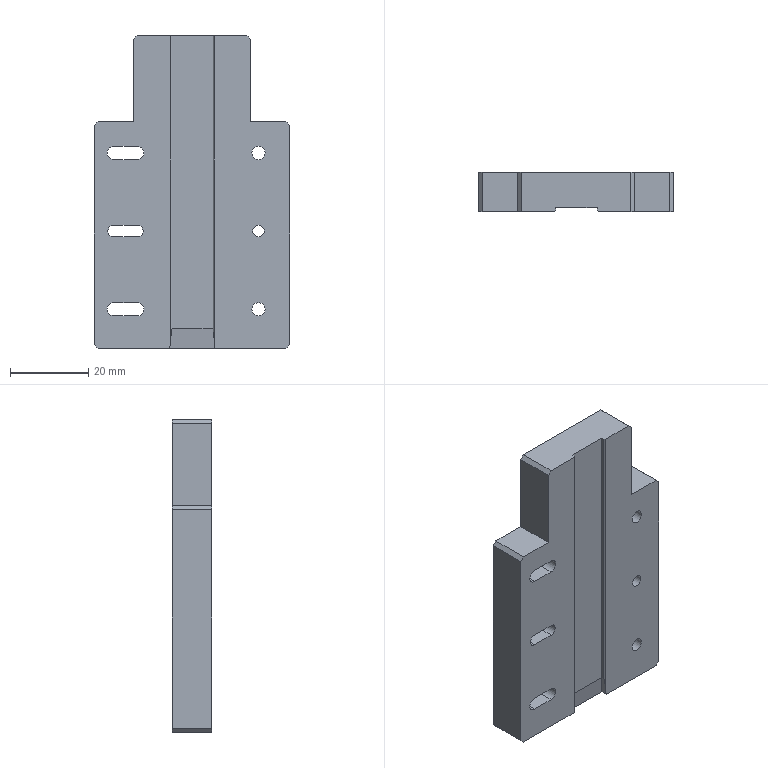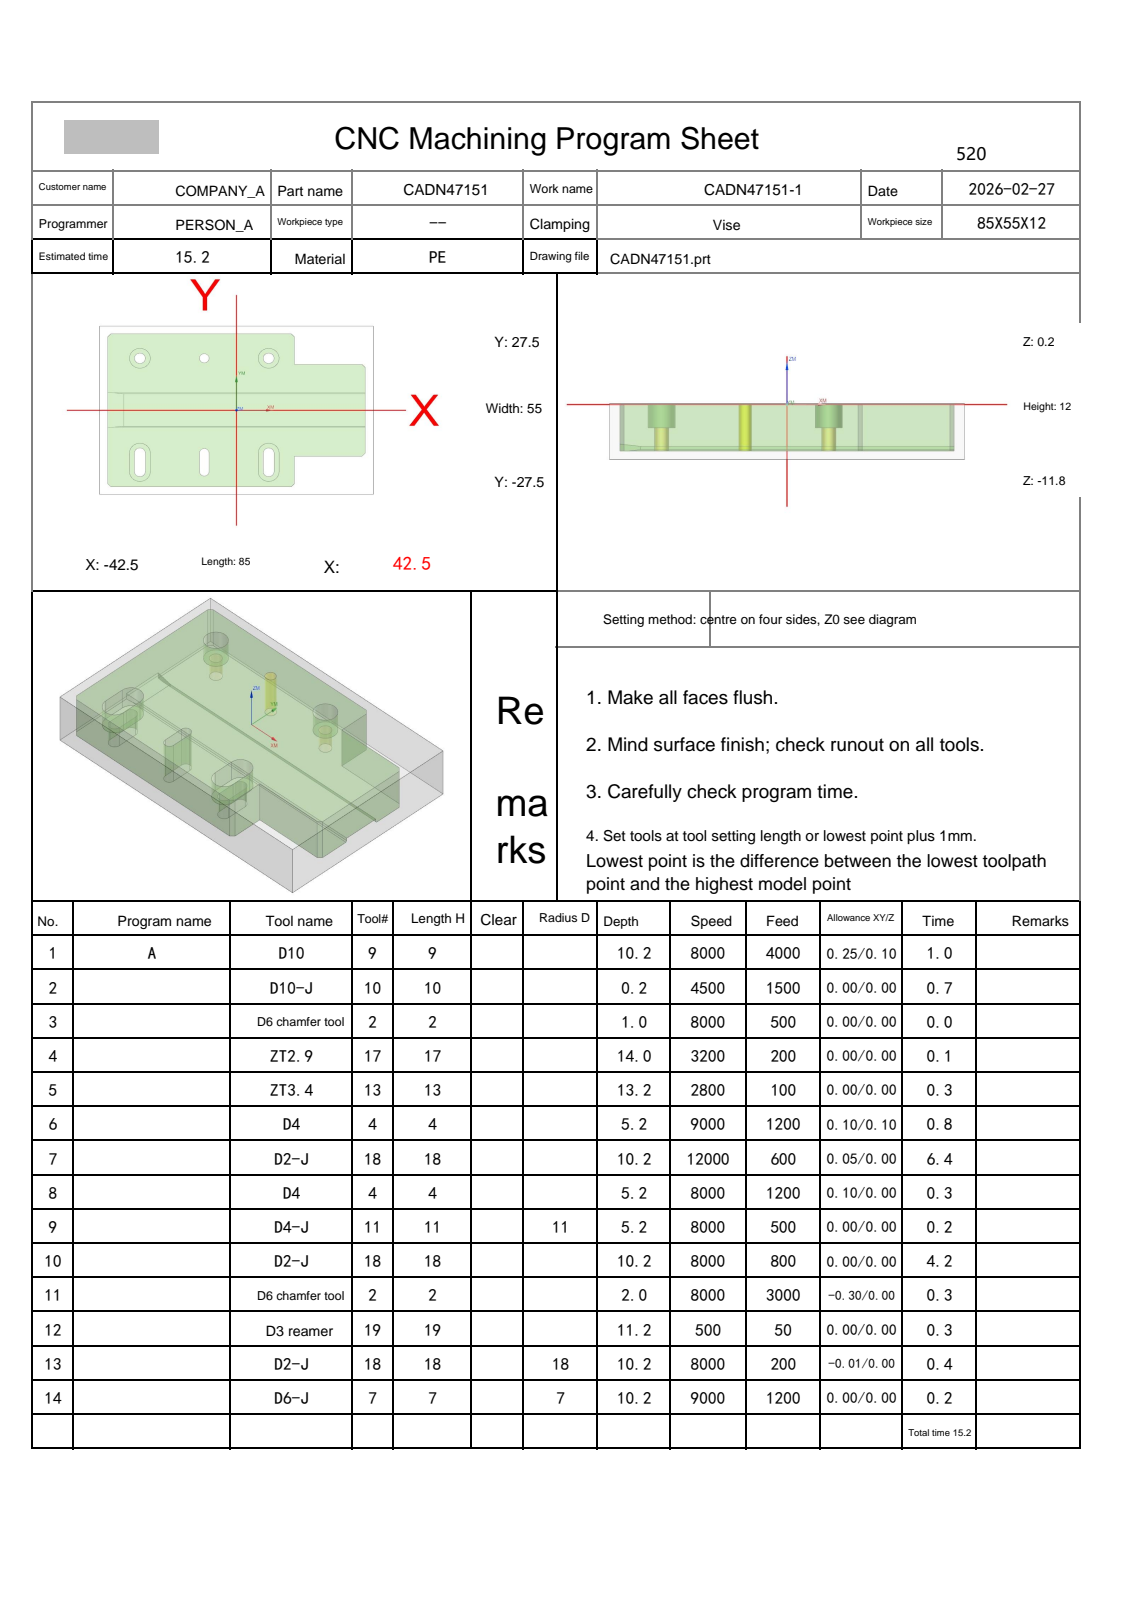NC program | NX | posted by the shop | part box 50 x 10 x 80 mm
Lines 1267 to 2934 of 8100, first 1180 of 1668 lines:
N7 T18 M06
(D2-J  D=2. R=0. H=18 ce=0.05 di=0.00)
G00 G90 G54 X-10.45 Y-17. M03 S12000
G43 H18 Z50.
M08
Z.5
G01 Y-20. Z.48 F600.
G03 X-10. Y-20.45 Z.475 I.45 J0.0
X-9.55 Y-20. Z.471 I0.0 J.45
G01 Y-14. Z.43
G03 X-10. Y-13.55 Z.426 I-.45 J0.0
X-10.45 Y-14. Z.421 I0.0 J-.45
G01 Y-20. Z.381
G03 X-10. Y-20.45 Z.376 I.45 J0.0
X-9.55 Y-20. Z.371 I0.0 J.45
G01 Y-14. Z.331
G03 X-10. Y-13.55 Z.327 I-.45 J0.0
X-10.45 Y-14. Z.322 I0.0 J-.45
G01 Y-20. Z.282
G03 X-10. Y-20.45 Z.277 I.45 J0.0
X-9.55 Y-20. Z.272 I0.0 J.45
G01 Y-14. Z.232
G03 X-10. Y-13.55 Z.228 I-.45 J0.0
X-10.45 Y-14. Z.223 I0.0 J-.45
G01 Y-20. Z.183
G03 X-10. Y-20.45 Z.178 I.45 J0.0
X-9.55 Y-20. Z.173 I0.0 J.45
G01 Y-14. Z.133
G03 X-10. Y-13.55 Z.129 I-.45 J0.0
X-10.45 Y-14. Z.124 I0.0 J-.45
G01 Y-20. Z.084
G03 X-10. Y-20.45 Z.079 I.45 J0.0
X-9.55 Y-20. Z.074 I0.0 J.45
G01 Y-14. Z.034
G03 X-10. Y-13.55 Z.029 I-.45 J0.0
X-10.45 Y-14. Z.025 I0.0 J-.45
G01 Y-20. Z-.015
G03 X-10. Y-20.45 Z-.02 I.45 J0.0
X-9.55 Y-20. Z-.025 I0.0 J.45
G01 Y-14. Z-.065
G03 X-10. Y-13.55 Z-.07 I-.45 J0.0
X-10.45 Y-14. Z-.074 I0.0 J-.45
G01 Y-20. Z-.114
G03 X-10. Y-20.45 Z-.119 I.45 J0.0
X-9.55 Y-20. Z-.124 I0.0 J.45
G01 Y-14. Z-.164
G03 X-10. Y-13.55 Z-.169 I-.45 J0.0
X-10.45 Y-14. Z-.173 I0.0 J-.45
G01 Y-20. Z-.213
G03 X-10. Y-20.45 Z-.218 I.45 J0.0
X-9.55 Y-20. Z-.223 I0.0 J.45
G01 Y-14. Z-.263
G03 X-10. Y-13.55 Z-.268 I-.45 J0.0
X-10.45 Y-14. Z-.272 I0.0 J-.45
G01 Y-20. Z-.312
G03 X-10. Y-20.45 Z-.317 I.45 J0.0
X-9.55 Y-20. Z-.322 I0.0 J.45
G01 Y-14. Z-.362
G03 X-10. Y-13.55 Z-.367 I-.45 J0.0
X-10.45 Y-14. Z-.371 I0.0 J-.45
G01 Y-20. Z-.412
G03 X-10. Y-20.45 Z-.416 I.45 J0.0
X-9.55 Y-20. Z-.421 I0.0 J.45
G01 Y-14. Z-.461
G03 X-10. Y-13.55 Z-.466 I-.45 J0.0
X-10.45 Y-14. Z-.471 I0.0 J-.45
G01 Y-20. Z-.511
G03 X-10. Y-20.45 Z-.515 I.45 J0.0
X-9.55 Y-20. Z-.52 I0.0 J.45
G01 Y-14. Z-.56
G03 X-10. Y-13.55 Z-.565 I-.45 J0.0
X-10.45 Y-14. Z-.57 I0.0 J-.45
G01 Y-20. Z-.61
G03 X-10. Y-20.45 Z-.614 I.45 J0.0
X-9.55 Y-20. Z-.619 I0.0 J.45
G01 Y-14. Z-.659
G03 X-10. Y-13.55 Z-.664 I-.45 J0.0
X-10.45 Y-14. Z-.669 I0.0 J-.45
G01 Y-20. Z-.709
G03 X-10. Y-20.45 Z-.713 I.45 J0.0
X-9.55 Y-20. Z-.718 I0.0 J.45
G01 Y-14. Z-.758
G03 X-10. Y-13.55 Z-.763 I-.45 J0.0
X-10.45 Y-14. Z-.768 I0.0 J-.45
G01 Y-20. Z-.808
G03 X-10. Y-20.45 Z-.813 I.45 J0.0
X-9.55 Y-20. Z-.817 I0.0 J.45
G01 Y-14. Z-.857
G03 X-10. Y-13.55 Z-.862 I-.45 J0.0
X-10.45 Y-14. Z-.867 I0.0 J-.45
G01 Y-20. Z-.907
G03 X-10. Y-20.45 Z-.912 I.45 J0.0
X-9.55 Y-20. Z-.916 I0.0 J.45
G01 Y-14. Z-.956
G03 X-10. Y-13.55 Z-.961 I-.45 J0.0
X-10.45 Y-14. Z-.966 I0.0 J-.45
G01 Y-20. Z-1.006
G03 X-10. Y-20.45 Z-1.011 I.45 J0.0
X-9.55 Y-20. Z-1.015 I0.0 J.45
G01 Y-14. Z-1.055
G03 X-10. Y-13.55 Z-1.06 I-.45 J0.0
X-10.45 Y-14. Z-1.065 I0.0 J-.45
G01 Y-20. Z-1.105
G03 X-10. Y-20.45 Z-1.11 I.45 J0.0
X-9.55 Y-20. Z-1.114 I0.0 J.45
G01 Y-14. Z-1.154
G03 X-10. Y-13.55 Z-1.159 I-.45 J0.0
X-10.45 Y-14. Z-1.164 I0.0 J-.45
G01 Y-20. Z-1.204
G03 X-10. Y-20.45 Z-1.209 I.45 J0.0
X-9.55 Y-20. Z-1.213 I0.0 J.45
G01 Y-14. Z-1.254
G03 X-10. Y-13.55 Z-1.258 I-.45 J0.0
X-10.45 Y-14. Z-1.263 I0.0 J-.45
G01 Y-20. Z-1.303
G03 X-10. Y-20.45 Z-1.308 I.45 J0.0
X-9.55 Y-20. Z-1.313 I0.0 J.45
G01 Y-14. Z-1.353
G03 X-10. Y-13.55 Z-1.357 I-.45 J0.0
X-10.45 Y-14. Z-1.362 I0.0 J-.45
G01 Y-20. Z-1.402
G03 X-10. Y-20.45 Z-1.407 I.45 J0.0
X-9.55 Y-20. Z-1.412 I0.0 J.45
G01 Y-14. Z-1.452
G03 X-10. Y-13.55 Z-1.456 I-.45 J0.0
X-10.45 Y-14. Z-1.461 I0.0 J-.45
G01 Y-20. Z-1.501
G03 X-10. Y-20.45 Z-1.506 I.45 J0.0
X-9.55 Y-20. Z-1.511 I0.0 J.45
G01 Y-14. Z-1.551
G03 X-10. Y-13.55 Z-1.555 I-.45 J0.0
X-10.45 Y-14. Z-1.56 I0.0 J-.45
G01 Y-20. Z-1.6
G03 X-10. Y-20.45 Z-1.605 I.45 J0.0
X-9.55 Y-20. Z-1.61 I0.0 J.45
G01 Y-14. Z-1.65
G03 X-10. Y-13.55 Z-1.654 I-.45 J0.0
X-10.45 Y-14. Z-1.659 I0.0 J-.45
G01 Y-20. Z-1.699
G03 X-10. Y-20.45 Z-1.704 I.45 J0.0
X-9.55 Y-20. Z-1.709 I0.0 J.45
G01 Y-14. Z-1.749
G03 X-10. Y-13.55 Z-1.754 I-.45 J0.0
X-10.45 Y-14. Z-1.758 I0.0 J-.45
G01 Y-20. Z-1.798
G03 X-10. Y-20.45 Z-1.803 I.45 J0.0
X-9.55 Y-20. Z-1.808 I0.0 J.45
G01 Y-14. Z-1.848
G03 X-10. Y-13.55 Z-1.853 I-.45 J0.0
X-10.45 Y-14. Z-1.857 I0.0 J-.45
G01 Y-20. Z-1.897
G03 X-10. Y-20.45 Z-1.902 I.45 J0.0
X-9.55 Y-20. Z-1.907 I0.0 J.45
G01 Y-14. Z-1.947
G03 X-10. Y-13.55 Z-1.952 I-.45 J0.0
X-10.45 Y-14. Z-1.956 I0.0 J-.45
G01 Y-20. Z-1.996
G03 X-10. Y-20.45 Z-2.001 I.45 J0.0
X-9.55 Y-20. Z-2.006 I0.0 J.45
G01 Y-14. Z-2.046
G03 X-10. Y-13.55 Z-2.051 I-.45 J0.0
X-10.45 Y-14. Z-2.055 I0.0 J-.45
G01 Y-20. Z-2.096
G03 X-10. Y-20.45 Z-2.1 I.45 J0.0
X-9.55 Y-20. Z-2.105 I0.0 J.45
G01 Y-14. Z-2.145
G03 X-10. Y-13.55 Z-2.15 I-.45 J0.0
X-10.45 Y-14. Z-2.154 I0.0 J-.45
G01 Y-20. Z-2.195
G03 X-10. Y-20.45 Z-2.199 I.45 J0.0
X-9.55 Y-20. Z-2.204 I0.0 J.45
G01 Y-14. Z-2.244
G03 X-10. Y-13.55 Z-2.249 I-.45 J0.0
X-10.45 Y-14. Z-2.254 I0.0 J-.45
G01 Y-20. Z-2.294
G03 X-10. Y-20.45 Z-2.298 I.45 J0.0
X-9.55 Y-20. Z-2.303 I0.0 J.45
G01 Y-14. Z-2.343
G03 X-10. Y-13.55 Z-2.348 I-.45 J0.0
X-10.45 Y-14. Z-2.353 I0.0 J-.45
G01 Y-20. Z-2.393
G03 X-10. Y-20.45 Z-2.397 I.45 J0.0
X-9.55 Y-20. Z-2.402 I0.0 J.45
G01 Y-14. Z-2.442
G03 X-10. Y-13.55 Z-2.447 I-.45 J0.0
X-10.45 Y-14. Z-2.452 I0.0 J-.45
G01 Y-20. Z-2.492
G03 X-10. Y-20.45 Z-2.496 I.45 J0.0
X-9.55 Y-20. Z-2.501 I0.0 J.45
G01 Y-14. Z-2.541
G03 X-10. Y-13.55 Z-2.546 I-.45 J0.0
X-10.45 Y-14. Z-2.551 I0.0 J-.45
G01 Y-20. Z-2.591
G03 X-10. Y-20.45 Z-2.596 I.45 J0.0
X-9.55 Y-20. Z-2.6 I0.0 J.45
G01 Y-14. Z-2.64
G03 X-10. Y-13.55 Z-2.645 I-.45 J0.0
X-10.45 Y-14. Z-2.65 I0.0 J-.45
G01 Y-20. Z-2.69
G03 X-10. Y-20.45 Z-2.695 I.45 J0.0
X-9.55 Y-20. Z-2.699 I0.0 J.45
G01 Y-14. Z-2.739
G03 X-10. Y-13.55 Z-2.744 I-.45 J0.0
X-10.45 Y-14. Z-2.749 I0.0 J-.45
G01 Y-20. Z-2.789
G03 X-10. Y-20.45 Z-2.794 I.45 J0.0
X-9.55 Y-20. Z-2.798 I0.0 J.45
G01 Y-14. Z-2.838
G03 X-10. Y-13.55 Z-2.843 I-.45 J0.0
X-10.45 Y-14. Z-2.848 I0.0 J-.45
G01 Y-20. Z-2.888
G03 X-10. Y-20.45 Z-2.893 I.45 J0.0
X-9.55 Y-20. Z-2.897 I0.0 J.45
G01 Y-14. Z-2.937
G03 X-10. Y-13.55 Z-2.942 I-.45 J0.0
X-10.45 Y-14. Z-2.947 I0.0 J-.45
G01 Y-20. Z-2.987
G03 X-10. Y-20.45 Z-2.992 I.45 J0.0
X-9.55 Y-20. Z-2.996 I0.0 J.45
G01 Y-14. Z-3.037
G03 X-10. Y-13.55 Z-3.041 I-.45 J0.0
X-10.45 Y-14. Z-3.046 I0.0 J-.45
G01 Y-20. Z-3.086
G03 X-10. Y-20.45 Z-3.091 I.45 J0.0
X-9.55 Y-20. Z-3.096 I0.0 J.45
G01 Y-14. Z-3.136
G03 X-10. Y-13.55 Z-3.14 I-.45 J0.0
X-10.45 Y-14. Z-3.145 I0.0 J-.45
G01 Y-20. Z-3.185
G03 X-10. Y-20.45 Z-3.19 I.45 J0.0
X-9.55 Y-20. Z-3.195 I0.0 J.45
G01 Y-14. Z-3.235
G03 X-10. Y-13.55 Z-3.239 I-.45 J0.0
X-10.45 Y-14. Z-3.244 I0.0 J-.45
G01 Y-20. Z-3.284
G03 X-10. Y-20.45 Z-3.289 I.45 J0.0
X-9.55 Y-20. Z-3.294 I0.0 J.45
G01 Y-14. Z-3.334
G03 X-10. Y-13.55 Z-3.338 I-.45 J0.0
X-10.45 Y-14. Z-3.343 I0.0 J-.45
G01 Y-20. Z-3.383
G03 X-10. Y-20.45 Z-3.388 I.45 J0.0
X-9.55 Y-20. Z-3.393 I0.0 J.45
G01 Y-14. Z-3.433
G03 X-10. Y-13.55 Z-3.438 I-.45 J0.0
X-10.45 Y-14. Z-3.442 I0.0 J-.45
G01 Y-20. Z-3.482
G03 X-10. Y-20.45 Z-3.487 I.45 J0.0
X-9.55 Y-20. Z-3.492 I0.0 J.45
G01 Y-14. Z-3.532
G03 X-10. Y-13.55 Z-3.537 I-.45 J0.0
X-10.45 Y-14. Z-3.541 I0.0 J-.45
G01 Y-20. Z-3.581
G03 X-10. Y-20.45 Z-3.586 I.45 J0.0
X-9.55 Y-20. Z-3.591 I0.0 J.45
G01 Y-14. Z-3.631
G03 X-10. Y-13.55 Z-3.636 I-.45 J0.0
X-10.45 Y-14. Z-3.64 I0.0 J-.45
G01 Y-20. Z-3.68
G03 X-10. Y-20.45 Z-3.685 I.45 J0.0
X-9.55 Y-20. Z-3.69 I0.0 J.45
G01 Y-14. Z-3.73
G03 X-10. Y-13.55 Z-3.735 I-.45 J0.0
X-10.45 Y-14. Z-3.739 I0.0 J-.45
G01 Y-20. Z-3.779
G03 X-10. Y-20.45 Z-3.784 I.45 J0.0
X-9.55 Y-20. Z-3.789 I0.0 J.45
G01 Y-14. Z-3.829
G03 X-10. Y-13.55 Z-3.834 I-.45 J0.0
X-10.45 Y-14. Z-3.838 I0.0 J-.45
G01 Y-20. Z-3.879
G03 X-10. Y-20.45 Z-3.883 I.45 J0.0
X-9.55 Y-20. Z-3.888 I0.0 J.45
G01 Y-14. Z-3.928
G03 X-10. Y-13.55 Z-3.933 I-.45 J0.0
X-10.45 Y-14. Z-3.938 I0.0 J-.45
G01 Y-20. Z-3.978
G03 X-10. Y-20.45 Z-3.982 I.45 J0.0
X-9.55 Y-20. Z-3.987 I0.0 J.45
G01 Y-14. Z-4.027
G03 X-10. Y-13.55 Z-4.032 I-.45 J0.0
X-10.45 Y-14. Z-4.037 I0.0 J-.45
G01 Y-20. Z-4.077
G03 X-10. Y-20.45 Z-4.081 I.45 J0.0
X-9.55 Y-20. Z-4.086 I0.0 J.45
G01 Y-14. Z-4.126
G03 X-10. Y-13.55 Z-4.131 I-.45 J0.0
X-10.45 Y-14. Z-4.136 I0.0 J-.45
G01 Y-20. Z-4.176
G03 X-10. Y-20.45 Z-4.18 I.45 J0.0
X-9.55 Y-20. Z-4.185 I0.0 J.45
G01 Y-14. Z-4.225
G03 X-10. Y-13.55 Z-4.23 I-.45 J0.0
X-10.45 Y-14. Z-4.235 I0.0 J-.45
G01 Y-20. Z-4.275
G03 X-10. Y-20.45 Z-4.279 I.45 J0.0
X-9.55 Y-20. Z-4.284 I0.0 J.45
G01 Y-14. Z-4.324
G03 X-10. Y-13.55 Z-4.329 I-.45 J0.0
X-10.45 Y-14. Z-4.334 I0.0 J-.45
G01 Y-20. Z-4.374
G03 X-10. Y-20.45 Z-4.379 I.45 J0.0
X-9.55 Y-20. Z-4.383 I0.0 J.45
G01 Y-14. Z-4.423
G03 X-10. Y-13.55 Z-4.428 I-.45 J0.0
X-10.45 Y-14. Z-4.433 I0.0 J-.45
G01 Y-20. Z-4.473
G03 X-10. Y-20.45 Z-4.478 I.45 J0.0
X-9.55 Y-20. Z-4.482 I0.0 J.45
G01 Y-14. Z-4.522
G03 X-10. Y-13.55 Z-4.527 I-.45 J0.0
X-10.45 Y-14. Z-4.532 I0.0 J-.45
G01 Y-20. Z-4.572
G03 X-10. Y-20.45 Z-4.577 I.45 J0.0
X-9.55 Y-20. Z-4.581 I0.0 J.45
G01 Y-14. Z-4.621
G03 X-10. Y-13.55 Z-4.626 I-.45 J0.0
X-10.45 Y-14. Z-4.631 I0.0 J-.45
G01 Y-20. Z-4.671
G03 X-10. Y-20.45 Z-4.676 I.45 J0.0
X-9.55 Y-20. Z-4.68 I0.0 J.45
G01 Y-14. Z-4.721
G03 X-10. Y-13.55 Z-4.725 I-.45 J0.0
X-10.45 Y-14. Z-4.73 I0.0 J-.45
G01 Y-20. Z-4.77
G03 X-10. Y-20.45 Z-4.775 I.45 J0.0
X-9.55 Y-20. Z-4.779 I0.0 J.45
G01 Y-14. Z-4.82
G03 X-10. Y-13.55 Z-4.824 I-.45 J0.0
X-10.45 Y-14. Z-4.829 I0.0 J-.45
G01 Y-20. Z-4.869
G03 X-10. Y-20.45 Z-4.874 I.45 J0.0
X-9.55 Y-20. Z-4.879 I0.0 J.45
G01 Y-14. Z-4.919
G03 X-10. Y-13.55 Z-4.923 I-.45 J0.0
X-10.45 Y-14. Z-4.928 I0.0 J-.45
G01 Y-20. Z-4.968
G03 X-10. Y-20.45 Z-4.973 I.45 J0.0
X-9.55 Y-20. Z-4.978 I0.0 J.45
G01 Y-14. Z-5.018
G03 X-10. Y-13.55 Z-5.022 I-.45 J0.0
X-10.45 Y-14. Z-5.027 I0.0 J-.45
G01 Y-20. Z-5.067
G03 X-10. Y-20.45 Z-5.072 I.45 J0.0
X-9.55 Y-20. Z-5.077 I0.0 J.45
G01 Y-14. Z-5.117
G03 X-10. Y-13.55 Z-5.121 I-.45 J0.0
X-10.45 Y-14. Z-5.126 I0.0 J-.45
G01 Y-20. Z-5.166
G03 X-10. Y-20.45 Z-5.171 I.45 J0.0
X-9.55 Y-20. Z-5.176 I0.0 J.45
G01 Y-14. Z-5.216
G03 X-10. Y-13.55 Z-5.221 I-.45 J0.0
X-10.45 Y-14. Z-5.225 I0.0 J-.45
G01 Y-20. Z-5.265
G03 X-10. Y-20.45 Z-5.27 I.45 J0.0
X-9.55 Y-20. Z-5.275 I0.0 J.45
G01 Y-14. Z-5.315
G03 X-10. Y-13.55 Z-5.32 I-.45 J0.0
X-10.45 Y-14. Z-5.324 I0.0 J-.45
G01 Y-20. Z-5.364
G03 X-10. Y-20.45 Z-5.369 I.45 J0.0
X-9.55 Y-20. Z-5.374 I0.0 J.45
G01 Y-14. Z-5.414
G03 X-10. Y-13.55 Z-5.419 I-.45 J0.0
X-10.45 Y-14. Z-5.423 I0.0 J-.45
G01 Y-20. Z-5.463
G03 X-10. Y-20.45 Z-5.468 I.45 J0.0
X-9.55 Y-20. Z-5.473 I0.0 J.45
G01 Y-14. Z-5.513
G03 X-10. Y-13.55 Z-5.518 I-.45 J0.0
X-10.45 Y-14. Z-5.522 I0.0 J-.45
G01 Y-20. Z-5.562
G03 X-10. Y-20.45 Z-5.567 I.45 J0.0
X-9.55 Y-20. Z-5.572 I0.0 J.45
G01 Y-14. Z-5.612
G03 X-10. Y-13.55 Z-5.617 I-.45 J0.0
X-10.45 Y-14. Z-5.621 I0.0 J-.45
G01 Y-20. Z-5.662
G03 X-10. Y-20.45 Z-5.666 I.45 J0.0
X-9.55 Y-20. Z-5.671 I0.0 J.45
G01 Y-14. Z-5.711
G03 X-10. Y-13.55 Z-5.716 I-.45 J0.0
X-10.45 Y-14. Z-5.721 I0.0 J-.45
G01 Y-20. Z-5.761
G03 X-10. Y-20.45 Z-5.765 I.45 J0.0
X-9.55 Y-20. Z-5.77 I0.0 J.45
G01 Y-14. Z-5.81
G03 X-10. Y-13.55 Z-5.815 I-.45 J0.0
X-10.45 Y-14. Z-5.82 I0.0 J-.45
G01 Y-20. Z-5.86
G03 X-10. Y-20.45 Z-5.864 I.45 J0.0
X-9.55 Y-20. Z-5.869 I0.0 J.45
G01 Y-14. Z-5.909
G03 X-10. Y-13.55 Z-5.914 I-.45 J0.0
X-10.45 Y-14. Z-5.919 I0.0 J-.45
G01 Y-20. Z-5.959
G03 X-10. Y-20.45 Z-5.963 I.45 J0.0
X-9.55 Y-20. Z-5.968 I0.0 J.45
G01 Y-14. Z-6.008
G03 X-10. Y-13.55 Z-6.013 I-.45 J0.0
X-10.45 Y-14. Z-6.018 I0.0 J-.45
G01 Y-20. Z-6.058
G03 X-10. Y-20.45 Z-6.063 I.45 J0.0
X-9.55 Y-20. Z-6.067 I0.0 J.45
G01 Y-14. Z-6.107
G03 X-10. Y-13.55 Z-6.112 I-.45 J0.0
X-10.45 Y-14. Z-6.117 I0.0 J-.45
G01 Y-20. Z-6.157
G03 X-10. Y-20.45 Z-6.162 I.45 J0.0
X-9.55 Y-20. Z-6.166 I0.0 J.45
G01 Y-14. Z-6.206
G03 X-10. Y-13.55 Z-6.211 I-.45 J0.0
X-10.45 Y-14. Z-6.216 I0.0 J-.45
G01 Y-20. Z-6.256
G03 X-10. Y-20.45 Z-6.261 I.45 J0.0
X-9.55 Y-20. Z-6.265 I0.0 J.45
G01 Y-14. Z-6.305
G03 X-10. Y-13.55 Z-6.31 I-.45 J0.0
X-10.45 Y-14. Z-6.315 I0.0 J-.45
G01 Y-20. Z-6.355
G03 X-10. Y-20.45 Z-6.36 I.45 J0.0
X-9.55 Y-20. Z-6.364 I0.0 J.45
G01 Y-14. Z-6.404
G03 X-10. Y-13.55 Z-6.409 I-.45 J0.0
X-10.45 Y-14. Z-6.414 I0.0 J-.45
G01 Y-20. Z-6.454
G03 X-10. Y-20.45 Z-6.459 I.45 J0.0
X-9.55 Y-20. Z-6.463 I0.0 J.45
G01 Y-14. Z-6.504
G03 X-10. Y-13.55 Z-6.508 I-.45 J0.0
X-10.45 Y-14. Z-6.513 I0.0 J-.45
G01 Y-20. Z-6.553
G03 X-10. Y-20.45 Z-6.558 I.45 J0.0
X-9.55 Y-20. Z-6.563 I0.0 J.45
G01 Y-14. Z-6.603
G03 X-10. Y-13.55 Z-6.607 I-.45 J0.0
X-10.45 Y-14. Z-6.612 I0.0 J-.45
G01 Y-20. Z-6.652
G03 X-10. Y-20.45 Z-6.657 I.45 J0.0
X-9.55 Y-20. Z-6.662 I0.0 J.45
G01 Y-14. Z-6.702
G03 X-10. Y-13.55 Z-6.706 I-.45 J0.0
X-10.45 Y-14. Z-6.711 I0.0 J-.45
G01 Y-20. Z-6.751
G03 X-10. Y-20.45 Z-6.756 I.45 J0.0
X-9.55 Y-20. Z-6.761 I0.0 J.45
G01 Y-14. Z-6.801
G03 X-10. Y-13.55 Z-6.805 I-.45 J0.0
X-10.45 Y-14. Z-6.81 I0.0 J-.45
G01 Y-20. Z-6.85
G03 X-10. Y-20.45 Z-6.855 I.45 J0.0
X-9.55 Y-20. Z-6.86 I0.0 J.45
G01 Y-14. Z-6.9
G03 X-10. Y-13.55 Z-6.904 I-.45 J0.0
X-10.45 Y-14. Z-6.909 I0.0 J-.45
G01 Y-20. Z-6.949
G03 X-10. Y-20.45 Z-6.954 I.45 J0.0
X-9.55 Y-20. Z-6.959 I0.0 J.45
G01 Y-14. Z-6.999
G03 X-10. Y-13.55 Z-7.004 I-.45 J0.0
X-10.45 Y-14. Z-7.008 I0.0 J-.45
G01 Y-20. Z-7.048
G03 X-10. Y-20.45 Z-7.053 I.45 J0.0
X-9.55 Y-20. Z-7.058 I0.0 J.45
G01 Y-14. Z-7.098
G03 X-10. Y-13.55 Z-7.103 I-.45 J0.0
X-10.45 Y-14. Z-7.107 I0.0 J-.45
G01 Y-20. Z-7.147
G03 X-10. Y-20.45 Z-7.152 I.45 J0.0
X-9.55 Y-20. Z-7.157 I0.0 J.45
G01 Y-14. Z-7.197
G03 X-10. Y-13.55 Z-7.202 I-.45 J0.0
X-10.45 Y-14. Z-7.206 I0.0 J-.45
G01 Y-20. Z-7.246
G03 X-10. Y-20.45 Z-7.251 I.45 J0.0
X-9.55 Y-20. Z-7.256 I0.0 J.45
G01 Y-14. Z-7.296
G03 X-10. Y-13.55 Z-7.301 I-.45 J0.0
X-10.45 Y-14. Z-7.305 I0.0 J-.45
G01 Y-20. Z-7.346
G03 X-10. Y-20.45 Z-7.35 I.45 J0.0
X-9.55 Y-20. Z-7.355 I0.0 J.45
G01 Y-14. Z-7.395
G03 X-10. Y-13.55 Z-7.4 I-.45 J0.0
X-10.45 Y-14. Z-7.404 I0.0 J-.45
G01 Y-20. Z-7.445
G03 X-10. Y-20.45 Z-7.449 I.45 J0.0
X-9.55 Y-20. Z-7.454 I0.0 J.45
G01 Y-14. Z-7.494
G03 X-10. Y-13.55 Z-7.499 I-.45 J0.0
X-10.45 Y-14. Z-7.504 I0.0 J-.45
G01 Y-20. Z-7.544
G03 X-10. Y-20.45 Z-7.548 I.45 J0.0
X-9.55 Y-20. Z-7.553 I0.0 J.45
G01 Y-14. Z-7.593
G03 X-10. Y-13.55 Z-7.598 I-.45 J0.0
X-10.45 Y-14. Z-7.603 I0.0 J-.45
G01 Y-20. Z-7.643
G03 X-10. Y-20.45 Z-7.647 I.45 J0.0
X-9.55 Y-20. Z-7.652 I0.0 J.45
G01 Y-14. Z-7.692
G03 X-10. Y-13.55 Z-7.697 I-.45 J0.0
X-10.45 Y-14. Z-7.702 I0.0 J-.45
G01 Y-20. Z-7.742
G03 X-10. Y-20.45 Z-7.746 I.45 J0.0
X-9.55 Y-20. Z-7.751 I0.0 J.45
G01 Y-14. Z-7.791
G03 X-10. Y-13.55 Z-7.796 I-.45 J0.0
X-10.45 Y-14. Z-7.801 I0.0 J-.45
G01 Y-20. Z-7.841
G03 X-10. Y-20.45 Z-7.846 I.45 J0.0
X-9.55 Y-20. Z-7.85 I0.0 J.45
G01 Y-14. Z-7.89
G03 X-10. Y-13.55 Z-7.895 I-.45 J0.0
X-10.45 Y-14. Z-7.9 I0.0 J-.45
G01 Y-20. Z-7.94
G03 X-10. Y-20.45 Z-7.945 I.45 J0.0
X-9.55 Y-20. Z-7.949 I0.0 J.45
G01 Y-14. Z-7.989
G03 X-10. Y-13.55 Z-7.994 I-.45 J0.0
X-10.45 Y-14. Z-7.999 I0.0 J-.45
G01 Y-20. Z-8.039
G03 X-10. Y-20.45 Z-8.044 I.45 J0.0
X-9.55 Y-20. Z-8.048 I0.0 J.45
G01 Y-14. Z-8.088
G03 X-10. Y-13.55 Z-8.093 I-.45 J0.0
X-10.45 Y-14. Z-8.098 I0.0 J-.45
G01 Y-20. Z-8.138
G03 X-10. Y-20.45 Z-8.143 I.45 J0.0
X-9.55 Y-20. Z-8.147 I0.0 J.45
G01 Y-14. Z-8.187
G03 X-10. Y-13.55 Z-8.192 I-.45 J0.0
X-10.45 Y-14. Z-8.197 I0.0 J-.45
G01 Y-20. Z-8.237
G03 X-10. Y-20.45 Z-8.242 I.45 J0.0
X-9.55 Y-20. Z-8.246 I0.0 J.45
G01 Y-14. Z-8.287
G03 X-10. Y-13.55 Z-8.291 I-.45 J0.0
X-10.45 Y-14. Z-8.296 I0.0 J-.45
G01 Y-20. Z-8.336
G03 X-10. Y-20.45 Z-8.341 I.45 J0.0
X-9.55 Y-20. Z-8.346 I0.0 J.45
G01 Y-14. Z-8.386
G03 X-10. Y-13.55 Z-8.39 I-.45 J0.0
X-10.45 Y-14. Z-8.395 I0.0 J-.45
G01 Y-20. Z-8.435
G03 X-10. Y-20.45 Z-8.44 I.45 J0.0
X-9.55 Y-20. Z-8.445 I0.0 J.45
G01 Y-14. Z-8.485
G03 X-10. Y-13.55 Z-8.489 I-.45 J0.0
X-10.45 Y-14. Z-8.494 I0.0 J-.45
G01 Y-20. Z-8.534
G03 X-10. Y-20.45 Z-8.539 I.45 J0.0
X-9.55 Y-20. Z-8.544 I0.0 J.45
G01 Y-14. Z-8.584
G03 X-10. Y-13.55 Z-8.588 I-.45 J0.0
X-10.45 Y-14. Z-8.593 I0.0 J-.45
G01 Y-20. Z-8.633
G03 X-10. Y-20.45 Z-8.638 I.45 J0.0
X-9.55 Y-20. Z-8.643 I0.0 J.45
G01 Y-14. Z-8.683
G03 X-10. Y-13.55 Z-8.688 I-.45 J0.0
X-10.45 Y-14. Z-8.692 I0.0 J-.45
G01 Y-20. Z-8.732
G03 X-10. Y-20.45 Z-8.737 I.45 J0.0
X-9.55 Y-20. Z-8.742 I0.0 J.45
G01 Y-14. Z-8.782
G03 X-10. Y-13.55 Z-8.787 I-.45 J0.0
X-10.45 Y-14. Z-8.791 I0.0 J-.45
G01 Y-20. Z-8.831
G03 X-10. Y-20.45 Z-8.836 I.45 J0.0
X-9.55 Y-20. Z-8.841 I0.0 J.45
G01 Y-14. Z-8.881
G03 X-10. Y-13.55 Z-8.886 I-.45 J0.0
X-10.45 Y-14. Z-8.89 I0.0 J-.45
G01 Y-20. Z-8.93
G03 X-10. Y-20.45 Z-8.935 I.45 J0.0
X-9.55 Y-20. Z-8.94 I0.0 J.45
G01 Y-14. Z-8.98
G03 X-10. Y-13.55 Z-8.985 I-.45 J0.0
X-10.45 Y-14. Z-8.989 I0.0 J-.45
G01 Y-20. Z-9.029
G03 X-10. Y-20.45 Z-9.034 I.45 J0.0
X-9.55 Y-20. Z-9.039 I0.0 J.45
G01 Y-14. Z-9.079
G03 X-10. Y-13.55 Z-9.084 I-.45 J0.0
X-10.45 Y-14. Z-9.088 I0.0 J-.45
G01 Y-20. Z-9.129
G03 X-10. Y-20.45 Z-9.133 I.45 J0.0
X-9.55 Y-20. Z-9.138 I0.0 J.45
G01 Y-14. Z-9.178
G03 X-10. Y-13.55 Z-9.183 I-.45 J0.0
X-10.45 Y-14. Z-9.188 I0.0 J-.45
G01 Y-20. Z-9.228
G03 X-10. Y-20.45 Z-9.232 I.45 J0.0
X-9.55 Y-20. Z-9.237 I0.0 J.45
G01 Y-14. Z-9.277
G03 X-10. Y-13.55 Z-9.282 I-.45 J0.0
X-10.45 Y-14. Z-9.287 I0.0 J-.45
G01 Y-20. Z-9.327
G03 X-10. Y-20.45 Z-9.331 I.45 J0.0
X-9.55 Y-20. Z-9.336 I0.0 J.45
G01 Y-14. Z-9.376
G03 X-10. Y-13.55 Z-9.381 I-.45 J0.0
X-10.45 Y-14. Z-9.386 I0.0 J-.45
G01 Y-20. Z-9.426
G03 X-10. Y-20.45 Z-9.43 I.45 J0.0
X-9.55 Y-20. Z-9.435 I0.0 J.45
G01 Y-14. Z-9.475
G03 X-10. Y-13.55 Z-9.48 I-.45 J0.0
X-10.45 Y-14. Z-9.485 I0.0 J-.45
G01 Y-20. Z-9.525
G03 X-10. Y-20.45 Z-9.529 I.45 J0.0
X-9.55 Y-20. Z-9.534 I0.0 J.45
G01 Y-14. Z-9.574
G03 X-10. Y-13.55 Z-9.579 I-.45 J0.0
X-10.45 Y-14. Z-9.584 I0.0 J-.45
G01 Y-20. Z-9.624
G03 X-10. Y-20.45 Z-9.629 I.45 J0.0
X-9.55 Y-20. Z-9.633 I0.0 J.45
G01 Y-14. Z-9.673
G03 X-10. Y-13.55 Z-9.678 I-.45 J0.0
X-10.45 Y-14. Z-9.683 I0.0 J-.45
G01 Y-20. Z-9.723
G03 X-10. Y-20.45 Z-9.728 I.45 J0.0
X-9.55 Y-20. Z-9.732 I0.0 J.45
G01 Y-14. Z-9.772
G03 X-10. Y-13.55 Z-9.777 I-.45 J0.0
X-10.45 Y-14. Z-9.782 I0.0 J-.45
G01 Y-20. Z-9.822
G03 X-10. Y-20.45 Z-9.827 I.45 J0.0
X-9.55 Y-20. Z-9.831 I0.0 J.45
G01 Y-14. Z-9.871
G03 X-10. Y-13.55 Z-9.876 I-.45 J0.0
X-10.45 Y-14. Z-9.881 I0.0 J-.45
G01 Y-20. Z-9.921
G03 X-10. Y-20.45 Z-9.926 I.45 J0.0
X-9.55 Y-20. Z-9.93 I0.0 J.45
G01 Y-14. Z-9.971
G03 X-10. Y-13.55 Z-9.975 I-.45 J0.0
X-10.45 Y-14. Z-9.98 I0.0 J-.45
G01 Y-17. Z-10.
Y-20.
G03 X-10. Y-20.45 I.45 J0.0
X-9.55 Y-20. I0.0 J.45
G01 Y-14.
G03 X-10. Y-13.55 I-.45 J0.0
X-10.45 Y-14. I0.0 J-.45
G01 Y-17.
Y-17.5
Z-9.
G00 Z50.
G00 G90 X-30.6 Y-17. M03 S12000
Z50.
Z-4.5
G01 Y-20. Z-4.515 F600.
G03 X-30. Y-20.6 Z-4.52 I.6 J0.0
X-29.4 Y-20. Z-4.525 I0.0 J.6
G01 Y-14. Z-4.555
G03 X-30. Y-13.4 Z-4.56 I-.6 J0.0
X-30.6 Y-14. Z-4.565 I0.0 J-.6
G01 Y-20. Z-4.595
G03 X-30. Y-20.6 Z-4.6 I.6 J0.0
X-29.4 Y-20. Z-4.604 I0.0 J.6
G01 Y-14. Z-4.635
G03 X-30. Y-13.4 Z-4.639 I-.6 J0.0
X-30.6 Y-14. Z-4.644 I0.0 J-.6
G01 Y-20. Z-4.675
G03 X-30. Y-20.6 Z-4.679 I.6 J0.0
X-29.4 Y-20. Z-4.684 I0.0 J.6
G01 Y-14. Z-4.714
G03 X-30. Y-13.4 Z-4.719 I-.6 J0.0
X-30.6 Y-14. Z-4.724 I0.0 J-.6
G01 Y-20. Z-4.754
G03 X-30. Y-20.6 Z-4.759 I.6 J0.0
X-29.4 Y-20. Z-4.764 I0.0 J.6
G01 Y-14. Z-4.794
G03 X-30. Y-13.4 Z-4.799 I-.6 J0.0
X-30.6 Y-14. Z-4.804 I0.0 J-.6
G01 Y-20. Z-4.834
G03 X-30. Y-20.6 Z-4.839 I.6 J0.0
X-29.4 Y-20. Z-4.844 I0.0 J.6
G01 Y-14. Z-4.874
G03 X-30. Y-13.4 Z-4.879 I-.6 J0.0
X-30.6 Y-14. Z-4.883 I0.0 J-.6
G01 Y-20. Z-4.914
G03 X-30. Y-20.6 Z-4.918 I.6 J0.0
X-29.4 Y-20. Z-4.923 I0.0 J.6
G01 Y-14. Z-4.954
G03 X-30. Y-13.4 Z-4.958 I-.6 J0.0
X-30.6 Y-14. Z-4.963 I0.0 J-.6
G01 Y-20. Z-4.993
G03 X-30. Y-20.6 Z-4.998 I.6 J0.0
X-29.4 Y-20. Z-5.003 I0.0 J.6
G01 Y-14. Z-5.033
G03 X-30. Y-13.4 Z-5.038 I-.6 J0.0
X-30.6 Y-14. Z-5.043 I0.0 J-.6
G01 Y-20. Z-5.073
G03 X-30. Y-20.6 Z-5.078 I.6 J0.0
X-29.4 Y-20. Z-5.083 I0.0 J.6
G01 Y-14. Z-5.113
G03 X-30. Y-13.4 Z-5.118 I-.6 J0.0
X-30.6 Y-14. Z-5.123 I0.0 J-.6
G01 Y-20. Z-5.153
G03 X-30. Y-20.6 Z-5.158 I.6 J0.0
X-29.4 Y-20. Z-5.162 I0.0 J.6
G01 Y-14. Z-5.193
G03 X-30. Y-13.4 Z-5.197 I-.6 J0.0
X-30.6 Y-14. Z-5.202 I0.0 J-.6
G01 Y-20. Z-5.233
G03 X-30. Y-20.6 Z-5.237 I.6 J0.0
X-29.4 Y-20. Z-5.242 I0.0 J.6
G01 Y-14. Z-5.272
G03 X-30. Y-13.4 Z-5.277 I-.6 J0.0
X-30.6 Y-14. Z-5.282 I0.0 J-.6
G01 Y-20. Z-5.312
G03 X-30. Y-20.6 Z-5.317 I.6 J0.0
X-29.4 Y-20. Z-5.322 I0.0 J.6
G01 Y-14. Z-5.352
G03 X-30. Y-13.4 Z-5.357 I-.6 J0.0
X-30.6 Y-14. Z-5.362 I0.0 J-.6
G01 Y-20. Z-5.392
G03 X-30. Y-20.6 Z-5.397 I.6 J0.0
X-29.4 Y-20. Z-5.402 I0.0 J.6
G01 Y-14. Z-5.432
G03 X-30. Y-13.4 Z-5.437 I-.6 J0.0
X-30.6 Y-14. Z-5.441 I0.0 J-.6
G01 Y-20. Z-5.472
G03 X-30. Y-20.6 Z-5.476 I.6 J0.0
X-29.4 Y-20. Z-5.481 I0.0 J.6
G01 Y-14. Z-5.512
G03 X-30. Y-13.4 Z-5.516 I-.6 J0.0
X-30.6 Y-14. Z-5.521 I0.0 J-.6
G01 Y-20. Z-5.551
G03 X-30. Y-20.6 Z-5.556 I.6 J0.0
X-29.4 Y-20. Z-5.561 I0.0 J.6
G01 Y-14. Z-5.591
G03 X-30. Y-13.4 Z-5.596 I-.6 J0.0
X-30.6 Y-14. Z-5.601 I0.0 J-.6
G01 Y-20. Z-5.631
G03 X-30. Y-20.6 Z-5.636 I.6 J0.0
X-29.4 Y-20. Z-5.641 I0.0 J.6
G01 Y-14. Z-5.671
G03 X-30. Y-13.4 Z-5.676 I-.6 J0.0
X-30.6 Y-14. Z-5.68 I0.0 J-.6
G01 Y-20. Z-5.711
G03 X-30. Y-20.6 Z-5.716 I.6 J0.0
X-29.4 Y-20. Z-5.72 I0.0 J.6
G01 Y-14. Z-5.751
G03 X-30. Y-13.4 Z-5.755 I-.6 J0.0
X-30.6 Y-14. Z-5.76 I0.0 J-.6
G01 Y-20. Z-5.791
G03 X-30. Y-20.6 Z-5.795 I.6 J0.0
X-29.4 Y-20. Z-5.8 I0.0 J.6
G01 Y-14. Z-5.83
G03 X-30. Y-13.4 Z-5.835 I-.6 J0.0
X-30.6 Y-14. Z-5.84 I0.0 J-.6
G01 Y-20. Z-5.87
G03 X-30. Y-20.6 Z-5.875 I.6 J0.0
X-29.4 Y-20. Z-5.88 I0.0 J.6
G01 Y-14. Z-5.91
G03 X-30. Y-13.4 Z-5.915 I-.6 J0.0
X-30.6 Y-14. Z-5.92 I0.0 J-.6
G01 Y-20. Z-5.95
G03 X-30. Y-20.6 Z-5.955 I.6 J0.0
X-29.4 Y-20. Z-5.959 I0.0 J.6
G01 Y-14. Z-5.99
G03 X-30. Y-13.4 Z-5.995 I-.6 J0.0
X-30.6 Y-14. Z-5.999 I0.0 J-.6
G01 Y-20. Z-6.03
G03 X-30. Y-20.6 Z-6.034 I.6 J0.0
X-29.4 Y-20. Z-6.039 I0.0 J.6
G01 Y-14. Z-6.07
G03 X-30. Y-13.4 Z-6.074 I-.6 J0.0
X-30.6 Y-14. Z-6.079 I0.0 J-.6
G01 Y-20. Z-6.109
G03 X-30. Y-20.6 Z-6.114 I.6 J0.0
X-29.4 Y-20. Z-6.119 I0.0 J.6
G01 Y-14. Z-6.149
G03 X-30. Y-13.4 Z-6.154 I-.6 J0.0
X-30.6 Y-14. Z-6.159 I0.0 J-.6
G01 Y-20. Z-6.189
G03 X-30. Y-20.6 Z-6.194 I.6 J0.0
X-29.4 Y-20. Z-6.199 I0.0 J.6
G01 Y-14. Z-6.229
G03 X-30. Y-13.4 Z-6.234 I-.6 J0.0
X-30.6 Y-14. Z-6.238 I0.0 J-.6
G01 Y-20. Z-6.269
G03 X-30. Y-20.6 Z-6.274 I.6 J0.0
X-29.4 Y-20. Z-6.278 I0.0 J.6
G01 Y-14. Z-6.309
G03 X-30. Y-13.4 Z-6.313 I-.6 J0.0
X-30.6 Y-14. Z-6.318 I0.0 J-.6
G01 Y-20. Z-6.348
G03 X-30. Y-20.6 Z-6.353 I.6 J0.0
X-29.4 Y-20. Z-6.358 I0.0 J.6
G01 Y-14. Z-6.388
G03 X-30. Y-13.4 Z-6.393 I-.6 J0.0
X-30.6 Y-14. Z-6.398 I0.0 J-.6
G01 Y-20. Z-6.428
G03 X-30. Y-20.6 Z-6.433 I.6 J0.0
X-29.4 Y-20. Z-6.438 I0.0 J.6
G01 Y-14. Z-6.468
G03 X-30. Y-13.4 Z-6.473 I-.6 J0.0
X-30.6 Y-14. Z-6.478 I0.0 J-.6
G01 Y-20. Z-6.508
G03 X-30. Y-20.6 Z-6.513 I.6 J0.0
X-29.4 Y-20. Z-6.517 I0.0 J.6
G01 Y-14. Z-6.548
G03 X-30. Y-13.4 Z-6.553 I-.6 J0.0
X-30.6 Y-14. Z-6.557 I0.0 J-.6
G01 Y-20. Z-6.588
G03 X-30. Y-20.6 Z-6.592 I.6 J0.0
X-29.4 Y-20. Z-6.597 I0.0 J.6
G01 Y-14. Z-6.627
G03 X-30. Y-13.4 Z-6.632 I-.6 J0.0
X-30.6 Y-14. Z-6.637 I0.0 J-.6
G01 Y-20. Z-6.667
G03 X-30. Y-20.6 Z-6.672 I.6 J0.0
X-29.4 Y-20. Z-6.677 I0.0 J.6
G01 Y-14. Z-6.707
G03 X-30. Y-13.4 Z-6.712 I-.6 J0.0
X-30.6 Y-14. Z-6.717 I0.0 J-.6
G01 Y-20. Z-6.747
G03 X-30. Y-20.6 Z-6.752 I.6 J0.0
X-29.4 Y-20. Z-6.757 I0.0 J.6
G01 Y-14. Z-6.787
G03 X-30. Y-13.4 Z-6.792 I-.6 J0.0
X-30.6 Y-14. Z-6.796 I0.0 J-.6
G01 Y-20. Z-6.827
G03 X-30. Y-20.6 Z-6.832 I.6 J0.0
X-29.4 Y-20. Z-6.836 I0.0 J.6
G01 Y-14. Z-6.867
G03 X-30. Y-13.4 Z-6.871 I-.6 J0.0
X-30.6 Y-14. Z-6.876 I0.0 J-.6
G01 Y-20. Z-6.906
G03 X-30. Y-20.6 Z-6.911 I.6 J0.0
X-29.4 Y-20. Z-6.916 I0.0 J.6
G01 Y-14. Z-6.946
G03 X-30. Y-13.4 Z-6.951 I-.6 J0.0
X-30.6 Y-14. Z-6.956 I0.0 J-.6
G01 Y-20. Z-6.986
G03 X-30. Y-20.6 Z-6.991 I.6 J0.0
X-29.4 Y-20. Z-6.996 I0.0 J.6
G01 Y-14. Z-7.026
G03 X-30. Y-13.4 Z-7.031 I-.6 J0.0
X-30.6 Y-14. Z-7.036 I0.0 J-.6
G01 Y-20. Z-7.066
G03 X-30. Y-20.6 Z-7.071 I.6 J0.0
X-29.4 Y-20. Z-7.075 I0.0 J.6
G01 Y-14. Z-7.106
G03 X-30. Y-13.4 Z-7.111 I-.6 J0.0
X-30.6 Y-14. Z-7.115 I0.0 J-.6
G01 Y-20. Z-7.146
G03 X-30. Y-20.6 Z-7.15 I.6 J0.0
X-29.4 Y-20. Z-7.155 I0.0 J.6
G01 Y-14. Z-7.185
G03 X-30. Y-13.4 Z-7.19 I-.6 J0.0
X-30.6 Y-14. Z-7.195 I0.0 J-.6
G01 Y-20. Z-7.225
G03 X-30. Y-20.6 Z-7.23 I.6 J0.0
X-29.4 Y-20. Z-7.235 I0.0 J.6
G01 Y-14. Z-7.265
G03 X-30. Y-13.4 Z-7.27 I-.6 J0.0
X-30.6 Y-14. Z-7.275 I0.0 J-.6
G01 Y-20. Z-7.305
G03 X-30. Y-20.6 Z-7.31 I.6 J0.0
X-29.4 Y-20. Z-7.315 I0.0 J.6
G01 Y-14. Z-7.345
G03 X-30. Y-13.4 Z-7.35 I-.6 J0.0
X-30.6 Y-14. Z-7.354 I0.0 J-.6
G01 Y-20. Z-7.385
G03 X-30. Y-20.6 Z-7.389 I.6 J0.0
X-29.4 Y-20. Z-7.394 I0.0 J.6
G01 Y-14. Z-7.425
G03 X-30. Y-13.4 Z-7.429 I-.6 J0.0
X-30.6 Y-14. Z-7.434 I0.0 J-.6
G01 Y-20. Z-7.464
G03 X-30. Y-20.6 Z-7.469 I.6 J0.0
X-29.4 Y-20. Z-7.474 I0.0 J.6
G01 Y-14. Z-7.504
G03 X-30. Y-13.4 Z-7.509 I-.6 J0.0
X-30.6 Y-14. Z-7.514 I0.0 J-.6
G01 Y-20. Z-7.544
G03 X-30. Y-20.6 Z-7.549 I.6 J0.0
X-29.4 Y-20. Z-7.554 I0.0 J.6
G01 Y-14. Z-7.584
G03 X-30. Y-13.4 Z-7.589 I-.6 J0.0
X-30.6 Y-14. Z-7.594 I0.0 J-.6
G01 Y-20. Z-7.624
G03 X-30. Y-20.6 Z-7.629 I.6 J0.0
X-29.4 Y-20. Z-7.633 I0.0 J.6
G01 Y-14. Z-7.664
G03 X-30. Y-13.4 Z-7.668 I-.6 J0.0
X-30.6 Y-14. Z-7.673 I0.0 J-.6
G01 Y-20. Z-7.704
G03 X-30. Y-20.6 Z-7.708 I.6 J0.0
X-29.4 Y-20. Z-7.713 I0.0 J.6
G01 Y-14. Z-7.743
G03 X-30. Y-13.4 Z-7.748 I-.6 J0.0
X-30.6 Y-14. Z-7.753 I0.0 J-.6
G01 Y-20. Z-7.783
G03 X-30. Y-20.6 Z-7.788 I.6 J0.0
X-29.4 Y-20. Z-7.793 I0.0 J.6
G01 Y-14. Z-7.823
G03 X-30. Y-13.4 Z-7.828 I-.6 J0.0
X-30.6 Y-14. Z-7.833 I0.0 J-.6
G01 Y-20. Z-7.863
G03 X-30. Y-20.6 Z-7.868 I.6 J0.0
X-29.4 Y-20. Z-7.873 I0.0 J.6
G01 Y-14. Z-7.903
G03 X-30. Y-13.4 Z-7.908 I-.6 J0.0
X-30.6 Y-14. Z-7.912 I0.0 J-.6
G01 Y-20. Z-7.943
G03 X-30. Y-20.6 Z-7.947 I.6 J0.0
X-29.4 Y-20. Z-7.952 I0.0 J.6
G01 Y-14. Z-7.983
G03 X-30. Y-13.4 Z-7.987 I-.6 J0.0
X-30.6 Y-14. Z-7.992 I0.0 J-.6
G01 Y-20. Z-8.022
G03 X-30. Y-20.6 Z-8.027 I.6 J0.0
X-29.4 Y-20. Z-8.032 I0.0 J.6
G01 Y-14. Z-8.062
G03 X-30. Y-13.4 Z-8.067 I-.6 J0.0
X-30.6 Y-14. Z-8.072 I0.0 J-.6
G01 Y-20. Z-8.102
G03 X-30. Y-20.6 Z-8.107 I.6 J0.0
X-29.4 Y-20. Z-8.112 I0.0 J.6
G01 Y-14. Z-8.142
G03 X-30. Y-13.4 Z-8.147 I-.6 J0.0
X-30.6 Y-14. Z-8.152 I0.0 J-.6
G01 Y-20. Z-8.182
G03 X-30. Y-20.6 Z-8.187 I.6 J0.0
X-29.4 Y-20. Z-8.191 I0.0 J.6
G01 Y-14. Z-8.222
G03 X-30. Y-13.4 Z-8.226 I-.6 J0.0
X-30.6 Y-14. Z-8.231 I0.0 J-.6
G01 Y-20. Z-8.262
G03 X-30. Y-20.6 Z-8.266 I.6 J0.0
X-29.4 Y-20. Z-8.271 I0.0 J.6
G01 Y-14. Z-8.301
G03 X-30. Y-13.4 Z-8.306 I-.6 J0.0
X-30.6 Y-14. Z-8.311 I0.0 J-.6
G01 Y-20. Z-8.341
G03 X-30. Y-20.6 Z-8.346 I.6 J0.0
X-29.4 Y-20. Z-8.351 I0.0 J.6
G01 Y-14. Z-8.381
G03 X-30. Y-13.4 Z-8.386 I-.6 J0.0
X-30.6 Y-14. Z-8.391 I0.0 J-.6
G01 Y-20. Z-8.421
G03 X-30. Y-20.6 Z-8.426 I.6 J0.0
X-29.4 Y-20. Z-8.43 I0.0 J.6
G01 Y-14. Z-8.461
G03 X-30. Y-13.4 Z-8.466 I-.6 J0.0
X-30.6 Y-14. Z-8.47 I0.0 J-.6
G01 Y-20. Z-8.501
G03 X-30. Y-20.6 Z-8.505 I.6 J0.0
X-29.4 Y-20. Z-8.51 I0.0 J.6
G01 Y-14. Z-8.541
G03 X-30. Y-13.4 Z-8.545 I-.6 J0.0
X-30.6 Y-14. Z-8.55 I0.0 J-.6
G01 Y-20. Z-8.58
G03 X-30. Y-20.6 Z-8.585 I.6 J0.0
X-29.4 Y-20. Z-8.59 I0.0 J.6
G01 Y-14. Z-8.62
G03 X-30. Y-13.4 Z-8.625 I-.6 J0.0
X-30.6 Y-14. Z-8.63 I0.0 J-.6
G01 Y-20. Z-8.66
G03 X-30. Y-20.6 Z-8.665 I.6 J0.0
X-29.4 Y-20. Z-8.67 I0.0 J.6
G01 Y-14. Z-8.7
G03 X-30. Y-13.4 Z-8.705 I-.6 J0.0
X-30.6 Y-14. Z-8.709 I0.0 J-.6
G01 Y-20. Z-8.74
G03 X-30. Y-20.6 Z-8.745 I.6 J0.0
X-29.4 Y-20. Z-8.749 I0.0 J.6
G01 Y-14. Z-8.78
G03 X-30. Y-13.4 Z-8.784 I-.6 J0.0
X-30.6 Y-14. Z-8.789 I0.0 J-.6
G01 Y-20. Z-8.82
G03 X-30. Y-20.6 Z-8.824 I.6 J0.0
X-29.4 Y-20. Z-8.829 I0.0 J.6
G01 Y-14. Z-8.859
G03 X-30. Y-13.4 Z-8.864 I-.6 J0.0
X-30.6 Y-14. Z-8.869 I0.0 J-.6
G01 Y-20. Z-8.899
G03 X-30. Y-20.6 Z-8.904 I.6 J0.0
X-29.4 Y-20. Z-8.909 I0.0 J.6
G01 Y-14. Z-8.939
G03 X-30. Y-13.4 Z-8.944 I-.6 J0.0
X-30.6 Y-14. Z-8.949 I0.0 J-.6
G01 Y-20. Z-8.979
G03 X-30. Y-20.6 Z-8.984 I.6 J0.0
X-29.4 Y-20. Z-8.988 I0.0 J.6
G01 Y-14. Z-9.019
G03 X-30. Y-13.4 Z-9.024 I-.6 J0.0
X-30.6 Y-14. Z-9.028 I0.0 J-.6
G01 Y-20. Z-9.059
G03 X-30. Y-20.6 Z-9.063 I.6 J0.0
X-29.4 Y-20. Z-9.068 I0.0 J.6
G01 Y-14. Z-9.098
G03 X-30. Y-13.4 Z-9.103 I-.6 J0.0
X-30.6 Y-14. Z-9.108 I0.0 J-.6
G01 Y-20. Z-9.138
G03 X-30. Y-20.6 Z-9.143 I.6 J0.0
X-29.4 Y-20. Z-9.148 I0.0 J.6
G01 Y-14. Z-9.178
G03 X-30. Y-13.4 Z-9.183 I-.6 J0.0
X-30.6 Y-14. Z-9.188 I0.0 J-.6
G01 Y-20. Z-9.218
G03 X-30. Y-20.6 Z-9.223 I.6 J0.0
X-29.4 Y-20. Z-9.228 I0.0 J.6
G01 Y-14. Z-9.258
G03 X-30. Y-13.4 Z-9.263 I-.6 J0.0
X-30.6 Y-14. Z-9.267 I0.0 J-.6
G01 Y-20. Z-9.298
G03 X-30. Y-20.6 Z-9.303 I.6 J0.0
X-29.4 Y-20. Z-9.307 I0.0 J.6
G01 Y-14. Z-9.338
G03 X-30. Y-13.4 Z-9.342 I-.6 J0.0
X-30.6 Y-14. Z-9.347 I0.0 J-.6
G01 Y-20. Z-9.377
G03 X-30. Y-20.6 Z-9.382 I.6 J0.0
X-29.4 Y-20. Z-9.387 I0.0 J.6
G01 Y-14. Z-9.417
G03 X-30. Y-13.4 Z-9.422 I-.6 J0.0
X-30.6 Y-14. Z-9.427 I0.0 J-.6
G01 Y-20. Z-9.457
G03 X-30. Y-20.6 Z-9.462 I.6 J0.0
X-29.4 Y-20. Z-9.467 I0.0 J.6
G01 Y-14. Z-9.497
G03 X-30. Y-13.4 Z-9.502 I-.6 J0.0
X-30.6 Y-14. Z-9.507 I0.0 J-.6
G01 Y-20. Z-9.537
G03 X-30. Y-20.6 Z-9.542 I.6 J0.0
X-29.4 Y-20. Z-9.546 I0.0 J.6
G01 Y-14. Z-9.577
G03 X-30. Y-13.4 Z-9.582 I-.6 J0.0
X-30.6 Y-14. Z-9.586 I0.0 J-.6
G01 Y-20. Z-9.617
G03 X-30. Y-20.6 Z-9.621 I.6 J0.0
X-29.4 Y-20. Z-9.626 I0.0 J.6
G01 Y-14. Z-9.656
G03 X-30. Y-13.4 Z-9.661 I-.6 J0.0
X-30.6 Y-14. Z-9.666 I0.0 J-.6
G01 Y-20. Z-9.696
G03 X-30. Y-20.6 Z-9.701 I.6 J0.0
X-29.4 Y-20. Z-9.706 I0.0 J.6
G01 Y-14. Z-9.736
G03 X-30. Y-13.4 Z-9.741 I-.6 J0.0
X-30.6 Y-14. Z-9.746 I0.0 J-.6
G01 Y-20. Z-9.776
G03 X-30. Y-20.6 Z-9.781 I.6 J0.0
X-29.4 Y-20. Z-9.786 I0.0 J.6
G01 Y-14. Z-9.816
G03 X-30. Y-13.4 Z-9.821 I-.6 J0.0
X-30.6 Y-14. Z-9.825 I0.0 J-.6
G01 Y-20. Z-9.856
G03 X-30. Y-20.6 Z-9.861 I.6 J0.0
X-29.4 Y-20. Z-9.865 I0.0 J.6
G01 Y-14. Z-9.896
G03 X-30. Y-13.4 Z-9.9 I-.6 J0.0
X-30.6 Y-14. Z-9.905 I0.0 J-.6
G01 Y-20. Z-9.935
G03 X-30. Y-20.6 Z-9.94 I.6 J0.0
X-29.4 Y-20. Z-9.945 I0.0 J.6
G01 Y-14. Z-9.975
G03 X-30. Y-13.4 Z-9.98 I-.6 J0.0
X-30.6 Y-14. Z-9.985 I0.0 J-.6
G01 Y-17. Z-10.
Y-20.
G03 X-30. Y-20.6 I.6 J0.0
X-29.4 Y-20. I0.0 J.6
G01 Y-14.
G03 X-30. Y-13.4 I-.6 J0.0
X-30.6 Y-14. I0.0 J-.6
G01 Y-17.
Y-17.5
Z-9.
G00 Z50.
X9.4 Y-17.
Z-4.5
G01 Y-20. Z-4.515
G03 X10. Y-20.6 Z-4.52 I.6 J0.0
X10.6 Y-20. Z-4.525 I0.0 J.6
G01 Y-14. Z-4.555
G03 X10. Y-13.4 Z-4.56 I-.6 J0.0
X9.4 Y-14. Z-4.565 I0.0 J-.6
G01 Y-20. Z-4.595
G03 X10. Y-20.6 Z-4.6 I.6 J0.0
X10.6 Y-20. Z-4.604 I0.0 J.6
G01 Y-14. Z-4.635
G03 X10. Y-13.4 Z-4.639 I-.6 J0.0
X9.4 Y-14. Z-4.644 I0.0 J-.6
G01 Y-20. Z-4.675
G03 X10. Y-20.6 Z-4.679 I.6 J0.0
X10.6 Y-20. Z-4.684 I0.0 J.6
G01 Y-14. Z-4.714
G03 X10. Y-13.4 Z-4.719 I-.6 J0.0
X9.4 Y-14. Z-4.724 I0.0 J-.6
G01 Y-20. Z-4.754
G03 X10. Y-20.6 Z-4.759 I.6 J0.0
X10.6 Y-20. Z-4.764 I0.0 J.6
G01 Y-14. Z-4.794
G03 X10. Y-13.4 Z-4.799 I-.6 J0.0
X9.4 Y-14. Z-4.804 I0.0 J-.6
G01 Y-20. Z-4.834
G03 X10. Y-20.6 Z-4.839 I.6 J0.0
X10.6 Y-20. Z-4.844 I0.0 J.6
G01 Y-14. Z-4.874
G03 X10. Y-13.4 Z-4.879 I-.6 J0.0
X9.4 Y-14. Z-4.883 I0.0 J-.6
G01 Y-20. Z-4.914
G03 X10. Y-20.6 Z-4.918 I.6 J0.0
X10.6 Y-20. Z-4.923 I0.0 J.6
G01 Y-14. Z-4.954
G03 X10. Y-13.4 Z-4.958 I-.6 J0.0
X9.4 Y-14. Z-4.963 I0.0 J-.6
G01 Y-20. Z-4.993
G03 X10. Y-20.6 Z-4.998 I.6 J0.0
X10.6 Y-20. Z-5.003 I0.0 J.6
G01 Y-14. Z-5.033
G03 X10. Y-13.4 Z-5.038 I-.6 J0.0
X9.4 Y-14. Z-5.043 I0.0 J-.6
G01 Y-20. Z-5.073
G03 X10. Y-20.6 Z-5.078 I.6 J0.0
X10.6 Y-20. Z-5.083 I0.0 J.6
G01 Y-14. Z-5.113
G03 X10. Y-13.4 Z-5.118 I-.6 J0.0
X9.4 Y-14. Z-5.123 I0.0 J-.6
G01 Y-20. Z-5.153
G03 X10. Y-20.6 Z-5.158 I.6 J0.0
X10.6 Y-20. Z-5.162 I0.0 J.6
G01 Y-14. Z-5.193
G03 X10. Y-13.4 Z-5.197 I-.6 J0.0
X9.4 Y-14. Z-5.202 I0.0 J-.6
G01 Y-20. Z-5.233
G03 X10. Y-20.6 Z-5.237 I.6 J0.0
X10.6 Y-20. Z-5.242 I0.0 J.6
G01 Y-14. Z-5.272
G03 X10. Y-13.4 Z-5.277 I-.6 J0.0
X9.4 Y-14. Z-5.282 I0.0 J-.6
G01 Y-20. Z-5.312
G03 X10. Y-20.6 Z-5.317 I.6 J0.0
X10.6 Y-20. Z-5.322 I0.0 J.6
G01 Y-14. Z-5.352
G03 X10. Y-13.4 Z-5.357 I-.6 J0.0
X9.4 Y-14. Z-5.362 I0.0 J-.6
G01 Y-20. Z-5.392
G03 X10. Y-20.6 Z-5.397 I.6 J0.0
X10.6 Y-20. Z-5.402 I0.0 J.6
G01 Y-14. Z-5.432
G03 X10. Y-13.4 Z-5.437 I-.6 J0.0
X9.4 Y-14. Z-5.441 I0.0 J-.6
G01 Y-20. Z-5.472
G03 X10. Y-20.6 Z-5.476 I.6 J0.0
X10.6 Y-20. Z-5.481 I0.0 J.6
G01 Y-14. Z-5.512
G03 X10. Y-13.4 Z-5.516 I-.6 J0.0
X9.4 Y-14. Z-5.521 I0.0 J-.6
G01 Y-20. Z-5.551
G03 X10. Y-20.6 Z-5.556 I.6 J0.0
X10.6 Y-20. Z-5.561 I0.0 J.6
G01 Y-14. Z-5.591
G03 X10. Y-13.4 Z-5.596 I-.6 J0.0
X9.4 Y-14. Z-5.601 I0.0 J-.6
G01 Y-20. Z-5.631
G03 X10. Y-20.6 Z-5.636 I.6 J0.0
X10.6 Y-20. Z-5.641 I0.0 J.6
G01 Y-14. Z-5.671
G03 X10. Y-13.4 Z-5.676 I-.6 J0.0
X9.4 Y-14. Z-5.68 I0.0 J-.6
G01 Y-20. Z-5.711
G03 X10. Y-20.6 Z-5.716 I.6 J0.0
X10.6 Y-20. Z-5.72 I0.0 J.6
G01 Y-14. Z-5.751
G03 X10. Y-13.4 Z-5.755 I-.6 J0.0
X9.4 Y-14. Z-5.76 I0.0 J-.6
G01 Y-20. Z-5.791